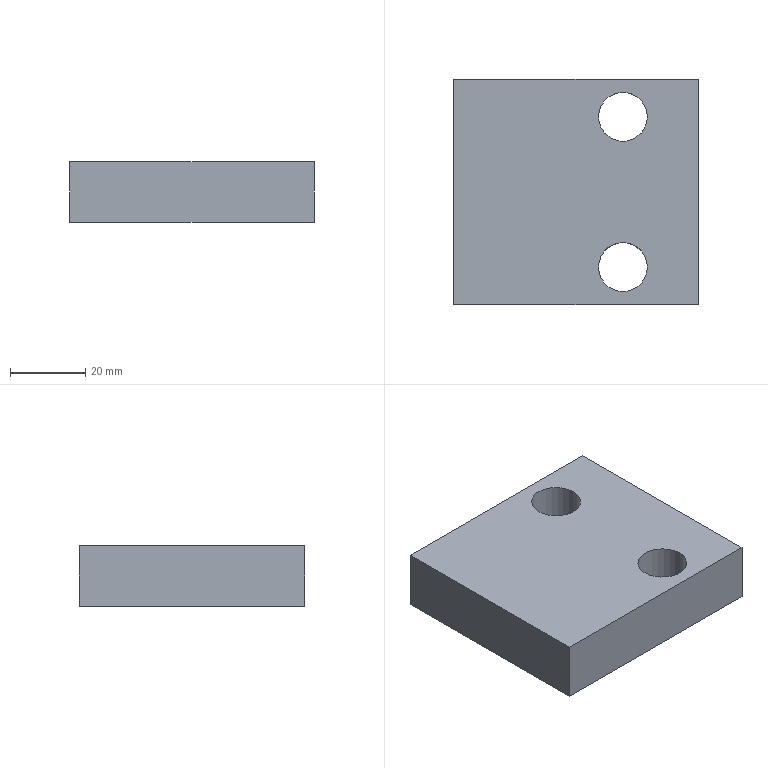Part | NX | features solid 2 | 1 solid | 8 faces | box 65 x 60 x 16 mm | volume 58153 mm3 | plane 6 | cylinder 2 | commonest cylinder face diameters 13 x2
STEP:
#1=CARTESIAN_POINT('',(753.5,-25.,81.));
#2=VERTEX_POINT('',#1);
#3=CARTESIAN_POINT('',(760.,-25.,81.));
#4=DIRECTION('',(0.,0.,-1.));
#5=DIRECTION('',(-1.,0.,0.));
#6=AXIS2_PLACEMENT_3D('',#3,#4,#5);
#7=CIRCLE('',#6,6.5);
#8=EDGE_CURVE('',#2,#2,#7,.F.);
#9=ORIENTED_EDGE('',*,*,#8,.F.);
#10=EDGE_LOOP('',(#9));
#11=FACE_BOUND('',#10,.T.);
#12=CARTESIAN_POINT('',(753.5,-65.,81.));
#13=VERTEX_POINT('',#12);
#14=CARTESIAN_POINT('',(760.,-65.,81.));
#15=DIRECTION('',(0.,0.,-1.));
#16=DIRECTION('',(-1.,0.,0.));
#17=AXIS2_PLACEMENT_3D('',#14,#15,#16);
#18=CIRCLE('',#17,6.5);
#19=EDGE_CURVE('',#13,#13,#18,.F.);
#20=ORIENTED_EDGE('',*,*,#19,.F.);
#21=EDGE_LOOP('',(#20));
#22=FACE_BOUND('',#21,.T.);
#23=CARTESIAN_POINT('',(715.,-75.,81.));
#24=VERTEX_POINT('',#23);
#25=CARTESIAN_POINT('',(780.,-75.,81.));
#26=VERTEX_POINT('',#25);
#27=CARTESIAN_POINT('',(730.,-75.,81.));
#28=DIRECTION('',(1.,0.,0.));
#29=VECTOR('',#28,1000.);
#30=LINE('',#27,#29);
#31=EDGE_CURVE('',#24,#26,#30,.T.);
#32=ORIENTED_EDGE('',*,*,#31,.T.);
#33=CARTESIAN_POINT('',(780.,-15.,81.));
#34=VERTEX_POINT('',#33);
#35=CARTESIAN_POINT('',(780.,-45.,81.));
#36=DIRECTION('',(0.,1.,0.));
#37=VECTOR('',#36,1000.);
#38=LINE('',#35,#37);
#39=EDGE_CURVE('',#26,#34,#38,.T.);
#40=ORIENTED_EDGE('',*,*,#39,.T.);
#41=CARTESIAN_POINT('',(715.,-15.,81.));
#42=VERTEX_POINT('',#41);
#43=CARTESIAN_POINT('',(730.,-15.,81.));
#44=DIRECTION('',(-1.,0.,0.));
#45=VECTOR('',#44,1000.);
#46=LINE('',#43,#45);
#47=EDGE_CURVE('',#34,#42,#46,.T.);
#48=ORIENTED_EDGE('',*,*,#47,.T.);
#49=CARTESIAN_POINT('',(715.,-45.,81.));
#50=DIRECTION('',(0.,-1.,0.));
#51=VECTOR('',#50,1000.);
#52=LINE('',#49,#51);
#53=EDGE_CURVE('',#42,#24,#52,.T.);
#54=ORIENTED_EDGE('',*,*,#53,.T.);
#55=EDGE_LOOP('',(#32,#40,#48,#54));
#56=FACE_BOUND('',#55,.T.);
#57=CARTESIAN_POINT('',(730.,-45.,81.));
#58=DIRECTION('',(0.,0.,1.));
#59=DIRECTION('',(-1.,0.,0.));
#60=AXIS2_PLACEMENT_3D('',#57,#58,#59);
#61=PLANE('',#60);
#62=ADVANCED_FACE('',(#11,#22,#56),#61,.T.);
#63=CARTESIAN_POINT('',(715.,-75.,65.));
#64=VERTEX_POINT('',#63);
#65=CARTESIAN_POINT('',(715.,-75.,65.));
#66=DIRECTION('',(0.,0.,1.));
#67=VECTOR('',#66,1000.);
#68=LINE('',#65,#67);
#69=EDGE_CURVE('',#64,#24,#68,.T.);
#70=ORIENTED_EDGE('',*,*,#69,.F.);
#71=CARTESIAN_POINT('',(780.,-75.,65.));
#72=VERTEX_POINT('',#71);
#73=CARTESIAN_POINT('',(730.,-75.,65.));
#74=DIRECTION('',(-1.,0.,0.));
#75=VECTOR('',#74,1000.);
#76=LINE('',#73,#75);
#77=EDGE_CURVE('',#72,#64,#76,.T.);
#78=ORIENTED_EDGE('',*,*,#77,.F.);
#79=CARTESIAN_POINT('',(780.,-75.,65.));
#80=DIRECTION('',(0.,0.,1.));
#81=VECTOR('',#80,1000.);
#82=LINE('',#79,#81);
#83=EDGE_CURVE('',#72,#26,#82,.T.);
#84=ORIENTED_EDGE('',*,*,#83,.T.);
#85=ORIENTED_EDGE('',*,*,#31,.F.);
#86=EDGE_LOOP('',(#70,#78,#84,#85));
#87=FACE_BOUND('',#86,.T.);
#88=CARTESIAN_POINT('',(730.,-75.,65.));
#89=DIRECTION('',(0.,-1.,0.));
#90=DIRECTION('',(0.,0.,-1.));
#91=AXIS2_PLACEMENT_3D('',#88,#89,#90);
#92=PLANE('',#91);
#93=ADVANCED_FACE('',(#87),#92,.T.);
#94=ORIENTED_EDGE('',*,*,#83,.F.);
#95=CARTESIAN_POINT('',(780.,-15.,65.));
#96=VERTEX_POINT('',#95);
#97=CARTESIAN_POINT('',(780.,-45.,65.));
#98=DIRECTION('',(0.,-1.,0.));
#99=VECTOR('',#98,1000.);
#100=LINE('',#97,#99);
#101=EDGE_CURVE('',#96,#72,#100,.T.);
#102=ORIENTED_EDGE('',*,*,#101,.F.);
#103=CARTESIAN_POINT('',(780.,-15.,65.));
#104=DIRECTION('',(0.,0.,1.));
#105=VECTOR('',#104,1000.);
#106=LINE('',#103,#105);
#107=EDGE_CURVE('',#96,#34,#106,.T.);
#108=ORIENTED_EDGE('',*,*,#107,.T.);
#109=ORIENTED_EDGE('',*,*,#39,.F.);
#110=EDGE_LOOP('',(#94,#102,#108,#109));
#111=FACE_BOUND('',#110,.T.);
#112=CARTESIAN_POINT('',(780.,-45.,65.));
#113=DIRECTION('',(1.,0.,0.));
#114=DIRECTION('',(0.,0.,1.));
#115=AXIS2_PLACEMENT_3D('',#112,#113,#114);
#116=PLANE('',#115);
#117=ADVANCED_FACE('',(#111),#116,.T.);
#118=ORIENTED_EDGE('',*,*,#107,.F.);
#119=CARTESIAN_POINT('',(715.,-15.,65.));
#120=VERTEX_POINT('',#119);
#121=CARTESIAN_POINT('',(730.,-15.,65.));
#122=DIRECTION('',(1.,0.,0.));
#123=VECTOR('',#122,1000.);
#124=LINE('',#121,#123);
#125=EDGE_CURVE('',#120,#96,#124,.T.);
#126=ORIENTED_EDGE('',*,*,#125,.F.);
#127=CARTESIAN_POINT('',(715.,-15.,65.));
#128=DIRECTION('',(0.,0.,1.));
#129=VECTOR('',#128,1000.);
#130=LINE('',#127,#129);
#131=EDGE_CURVE('',#120,#42,#130,.T.);
#132=ORIENTED_EDGE('',*,*,#131,.T.);
#133=ORIENTED_EDGE('',*,*,#47,.F.);
#134=EDGE_LOOP('',(#118,#126,#132,#133));
#135=FACE_BOUND('',#134,.T.);
#136=CARTESIAN_POINT('',(730.,-15.,65.));
#137=DIRECTION('',(0.,1.,0.));
#138=DIRECTION('',(0.,0.,1.));
#139=AXIS2_PLACEMENT_3D('',#136,#137,#138);
#140=PLANE('',#139);
#141=ADVANCED_FACE('',(#135),#140,.T.);
#142=CARTESIAN_POINT('',(766.5,-25.,65.));
#143=VERTEX_POINT('',#142);
#144=CARTESIAN_POINT('',(760.,-25.,65.));
#145=DIRECTION('',(0.,0.,1.));
#146=DIRECTION('',(1.,0.,0.));
#147=AXIS2_PLACEMENT_3D('',#144,#145,#146);
#148=CIRCLE('',#147,6.5);
#149=EDGE_CURVE('',#143,#143,#148,.T.);
#150=ORIENTED_EDGE('',*,*,#149,.T.);
#151=EDGE_LOOP('',(#150));
#152=FACE_BOUND('',#151,.T.);
#153=CARTESIAN_POINT('',(766.5,-65.,65.));
#154=VERTEX_POINT('',#153);
#155=CARTESIAN_POINT('',(760.,-65.,65.));
#156=DIRECTION('',(0.,0.,1.));
#157=DIRECTION('',(1.,0.,0.));
#158=AXIS2_PLACEMENT_3D('',#155,#156,#157);
#159=CIRCLE('',#158,6.5);
#160=EDGE_CURVE('',#154,#154,#159,.T.);
#161=ORIENTED_EDGE('',*,*,#160,.T.);
#162=EDGE_LOOP('',(#161));
#163=FACE_BOUND('',#162,.T.);
#164=CARTESIAN_POINT('',(715.,-45.,65.));
#165=DIRECTION('',(0.,1.,0.));
#166=VECTOR('',#165,1000.);
#167=LINE('',#164,#166);
#168=EDGE_CURVE('',#64,#120,#167,.T.);
#169=ORIENTED_EDGE('',*,*,#168,.T.);
#170=ORIENTED_EDGE('',*,*,#125,.T.);
#171=ORIENTED_EDGE('',*,*,#101,.T.);
#172=ORIENTED_EDGE('',*,*,#77,.T.);
#173=EDGE_LOOP('',(#169,#170,#171,#172));
#174=FACE_BOUND('',#173,.T.);
#175=CARTESIAN_POINT('',(730.,-45.,65.));
#176=DIRECTION('',(0.,0.,-1.));
#177=DIRECTION('',(1.,0.,0.));
#178=AXIS2_PLACEMENT_3D('',#175,#176,#177);
#179=PLANE('',#178);
#180=ADVANCED_FACE('',(#152,#163,#174),#179,.T.);
#181=ORIENTED_EDGE('',*,*,#168,.F.);
#182=ORIENTED_EDGE('',*,*,#69,.T.);
#183=ORIENTED_EDGE('',*,*,#53,.F.);
#184=ORIENTED_EDGE('',*,*,#131,.F.);
#185=EDGE_LOOP('',(#181,#182,#183,#184));
#186=FACE_BOUND('',#185,.T.);
#187=CARTESIAN_POINT('',(715.,-45.,65.));
#188=DIRECTION('',(-1.,0.,0.));
#189=DIRECTION('',(0.,0.,-1.));
#190=AXIS2_PLACEMENT_3D('',#187,#188,#189);
#191=PLANE('',#190);
#192=ADVANCED_FACE('',(#186),#191,.T.);
#193=ORIENTED_EDGE('',*,*,#160,.F.);
#194=EDGE_LOOP('',(#193));
#195=FACE_BOUND('',#194,.T.);
#196=ORIENTED_EDGE('',*,*,#19,.T.);
#197=EDGE_LOOP('',(#196));
#198=FACE_BOUND('',#197,.T.);
#199=CARTESIAN_POINT('',(760.,-65.,95.));
#200=DIRECTION('',(0.,0.,-1.));
#201=DIRECTION('',(0.,-1.,0.));
#202=AXIS2_PLACEMENT_3D('',#199,#200,#201);
#203=CYLINDRICAL_SURFACE('',#202,6.5);
#204=ADVANCED_FACE('',(#195,#198),#203,.F.);
#205=ORIENTED_EDGE('',*,*,#149,.F.);
#206=EDGE_LOOP('',(#205));
#207=FACE_BOUND('',#206,.T.);
#208=ORIENTED_EDGE('',*,*,#8,.T.);
#209=EDGE_LOOP('',(#208));
#210=FACE_BOUND('',#209,.T.);
#211=CARTESIAN_POINT('',(760.,-25.,95.));
#212=DIRECTION('',(0.,0.,-1.));
#213=DIRECTION('',(0.,-1.,0.));
#214=AXIS2_PLACEMENT_3D('',#211,#212,#213);
#215=CYLINDRICAL_SURFACE('',#214,6.5);
#216=ADVANCED_FACE('',(#207,#210),#215,.F.);
#217=CLOSED_SHELL('',(#62,#93,#117,#141,#180,#192,#204,#216));
#218=MANIFOLD_SOLID_BREP('',#217);
#219=(LENGTH_UNIT()NAMED_UNIT(*)SI_UNIT(.MILLI.,.METRE.));
#220=UNCERTAINTY_MEASURE_WITH_UNIT(LENGTH_MEASURE(0.00001),#219,'','');
#221=(NAMED_UNIT(*)PLANE_ANGLE_UNIT()SI_UNIT($,.RADIAN.));
#222=(NAMED_UNIT(*)SI_UNIT($,.STERADIAN.)SOLID_ANGLE_UNIT());
#223=(GEOMETRIC_REPRESENTATION_CONTEXT(3)GLOBAL_UNCERTAINTY_ASSIGNED_CONTEXT((#220))GLOBAL_UNIT_ASSIGNED_CONTEXT((#219,#221,#222))REPRESENTATION_CONTEXT('',''));
#224=ADVANCED_BREP_SHAPE_REPRESENTATION('',(#218),#223);